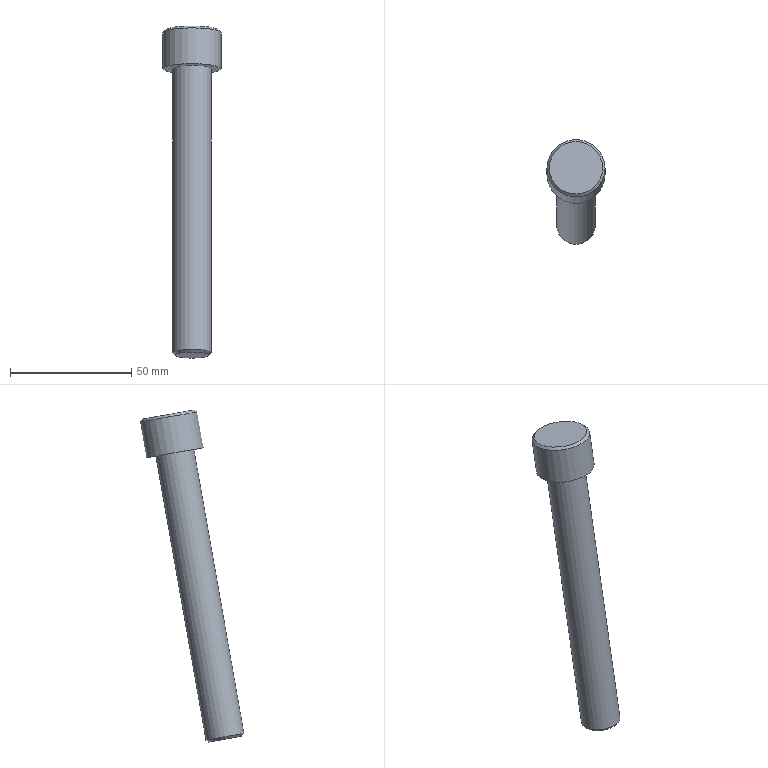Part | NX | features solid 2 | 1 solid | 7 faces | box 24 x 42.965 x 137.06 mm | volume 31305 mm3 | plane 3 | cylinder 2 | cone 2 | commonest cylinder face diameters 16 x1 24 x1
STEP:
#1=CARTESIAN_POINT('',(678.5,-825.645,152.223));
#2=VERTEX_POINT('',#1);
#3=CARTESIAN_POINT('',(666.5,-825.645,152.223));
#4=DIRECTION('',(0.,-0.1736,-0.9848));
#5=DIRECTION('',(1.,0.,0.));
#6=AXIS2_PLACEMENT_3D('',#3,#4,#5);
#7=CIRCLE('',#6,12.);
#8=EDGE_CURVE('',#2,#2,#7,.T.);
#9=ORIENTED_EDGE('',*,*,#8,.T.);
#10=EDGE_LOOP('',(#9));
#11=FACE_BOUND('',#10,.T.);
#12=CARTESIAN_POINT('',(674.5,-825.645,152.223));
#13=VERTEX_POINT('',#12);
#14=CARTESIAN_POINT('',(666.5,-825.645,152.223));
#15=DIRECTION('',(0.,-0.1736,-0.9848));
#16=DIRECTION('',(1.,0.,0.));
#17=AXIS2_PLACEMENT_3D('',#14,#15,#16);
#18=CIRCLE('',#17,8.);
#19=EDGE_CURVE('',#13,#13,#18,.F.);
#20=ORIENTED_EDGE('',*,*,#19,.T.);
#21=EDGE_LOOP('',(#20));
#22=FACE_BOUND('',#21,.T.);
#23=CARTESIAN_POINT('',(666.5,-825.645,152.223));
#24=DIRECTION('',(0.,0.1736,0.9848));
#25=DIRECTION('',(1.,0.,0.));
#26=AXIS2_PLACEMENT_3D('',#23,#24,#25);
#27=PLANE('',#26);
#28=ADVANCED_FACE('',(#11,#22),#27,.F.);
#29=CARTESIAN_POINT('',(678.5,-823.041,166.995));
#30=VERTEX_POINT('',#29);
#31=CARTESIAN_POINT('',(666.5,-823.041,166.995));
#32=DIRECTION('',(0.,-0.1736,-0.9848));
#33=DIRECTION('',(1.,0.,0.));
#34=AXIS2_PLACEMENT_3D('',#31,#32,#33);
#35=CIRCLE('',#34,12.);
#36=EDGE_CURVE('',#30,#30,#35,.F.);
#37=ORIENTED_EDGE('',*,*,#36,.F.);
#38=EDGE_LOOP('',(#37));
#39=FACE_BOUND('',#38,.T.);
#40=ORIENTED_EDGE('',*,*,#8,.F.);
#41=EDGE_LOOP('',(#40));
#42=FACE_BOUND('',#41,.T.);
#43=CARTESIAN_POINT('',(666.5,-814.184,217.22));
#44=DIRECTION('',(0.,-0.1736,-0.9848));
#45=DIRECTION('',(-1.,0.,0.));
#46=AXIS2_PLACEMENT_3D('',#43,#44,#45);
#47=CYLINDRICAL_SURFACE('',#46,12.);
#48=ADVANCED_FACE('',(#39,#42),#47,.T.);
#49=CARTESIAN_POINT('',(677.5,-822.867,167.98));
#50=VERTEX_POINT('',#49);
#51=CARTESIAN_POINT('',(666.5,-822.867,167.98));
#52=DIRECTION('',(0.,-0.1736,-0.9848));
#53=DIRECTION('',(1.,0.,0.));
#54=AXIS2_PLACEMENT_3D('',#51,#52,#53);
#55=CIRCLE('',#54,11.);
#56=EDGE_CURVE('',#50,#50,#55,.T.);
#57=ORIENTED_EDGE('',*,*,#56,.F.);
#58=EDGE_LOOP('',(#57));
#59=FACE_BOUND('',#58,.T.);
#60=CARTESIAN_POINT('',(666.5,-822.867,167.98));
#61=DIRECTION('',(0.,0.1736,0.9848));
#62=DIRECTION('',(1.,0.,0.));
#63=AXIS2_PLACEMENT_3D('',#60,#61,#62);
#64=PLANE('',#63);
#65=ADVANCED_FACE('',(#59),#64,.T.);
#66=CARTESIAN_POINT('',(674.5,-846.309,35.031));
#67=VERTEX_POINT('',#66);
#68=CARTESIAN_POINT('',(666.5,-846.309,35.031));
#69=DIRECTION('',(0.,-0.1736,-0.9848));
#70=DIRECTION('',(1.,0.,0.));
#71=AXIS2_PLACEMENT_3D('',#68,#69,#70);
#72=CIRCLE('',#71,8.);
#73=EDGE_CURVE('',#67,#67,#72,.T.);
#74=ORIENTED_EDGE('',*,*,#73,.F.);
#75=EDGE_LOOP('',(#74));
#76=FACE_BOUND('',#75,.T.);
#77=ORIENTED_EDGE('',*,*,#19,.F.);
#78=EDGE_LOOP('',(#77));
#79=FACE_BOUND('',#78,.T.);
#80=CARTESIAN_POINT('',(666.5,-816.963,201.463));
#81=DIRECTION('',(0.,-0.1736,-0.9848));
#82=DIRECTION('',(-1.,0.,0.));
#83=AXIS2_PLACEMENT_3D('',#80,#81,#82);
#84=CYLINDRICAL_SURFACE('',#83,8.);
#85=ADVANCED_FACE('',(#76,#79),#84,.T.);
#86=CARTESIAN_POINT('',(673.5,-846.483,34.046));
#87=VERTEX_POINT('',#86);
#88=CARTESIAN_POINT('',(666.5,-846.483,34.046));
#89=DIRECTION('',(0.,-0.1736,-0.9848));
#90=DIRECTION('',(1.,0.,0.));
#91=AXIS2_PLACEMENT_3D('',#88,#89,#90);
#92=CIRCLE('',#91,7.);
#93=EDGE_CURVE('',#87,#87,#92,.F.);
#94=ORIENTED_EDGE('',*,*,#93,.F.);
#95=EDGE_LOOP('',(#94));
#96=FACE_BOUND('',#95,.T.);
#97=CARTESIAN_POINT('',(666.5,-846.483,34.046));
#98=DIRECTION('',(0.,0.1736,0.9848));
#99=DIRECTION('',(1.,0.,0.));
#100=AXIS2_PLACEMENT_3D('',#97,#98,#99);
#101=PLANE('',#100);
#102=ADVANCED_FACE('',(#96),#101,.F.);
#103=ORIENTED_EDGE('',*,*,#93,.T.);
#104=EDGE_LOOP('',(#103));
#105=FACE_BOUND('',#104,.T.);
#106=ORIENTED_EDGE('',*,*,#73,.T.);
#107=EDGE_LOOP('',(#106));
#108=FACE_BOUND('',#107,.T.);
#109=CARTESIAN_POINT('',(666.5,-846.309,35.031));
#110=DIRECTION('',(0.,0.1736,0.9848));
#111=DIRECTION('',(1.,0.,0.));
#112=AXIS2_PLACEMENT_3D('',#109,#110,#111);
#113=CONICAL_SURFACE('',#112,8.,0.7854);
#114=ADVANCED_FACE('',(#105,#108),#113,.T.);
#115=ORIENTED_EDGE('',*,*,#36,.T.);
#116=EDGE_LOOP('',(#115));
#117=FACE_BOUND('',#116,.T.);
#118=ORIENTED_EDGE('',*,*,#56,.T.);
#119=EDGE_LOOP('',(#118));
#120=FACE_BOUND('',#119,.T.);
#121=CARTESIAN_POINT('',(666.5,-822.867,167.98));
#122=DIRECTION('',(0.,-0.1736,-0.9848));
#123=DIRECTION('',(-1.,0.,0.));
#124=AXIS2_PLACEMENT_3D('',#121,#122,#123);
#125=CONICAL_SURFACE('',#124,11.,0.7854);
#126=ADVANCED_FACE('',(#117,#120),#125,.T.);
#127=CLOSED_SHELL('',(#28,#48,#65,#85,#102,#114,#126));
#128=MANIFOLD_SOLID_BREP('',#127);
#129=(LENGTH_UNIT()NAMED_UNIT(*)SI_UNIT(.MILLI.,.METRE.));
#130=UNCERTAINTY_MEASURE_WITH_UNIT(LENGTH_MEASURE(0.00001),#129,'','');
#131=(NAMED_UNIT(*)PLANE_ANGLE_UNIT()SI_UNIT($,.RADIAN.));
#132=(NAMED_UNIT(*)SI_UNIT($,.STERADIAN.)SOLID_ANGLE_UNIT());
#133=(GEOMETRIC_REPRESENTATION_CONTEXT(3)GLOBAL_UNCERTAINTY_ASSIGNED_CONTEXT((#130))GLOBAL_UNIT_ASSIGNED_CONTEXT((#129,#131,#132))REPRESENTATION_CONTEXT('',''));
#134=ADVANCED_BREP_SHAPE_REPRESENTATION('',(#128),#133);